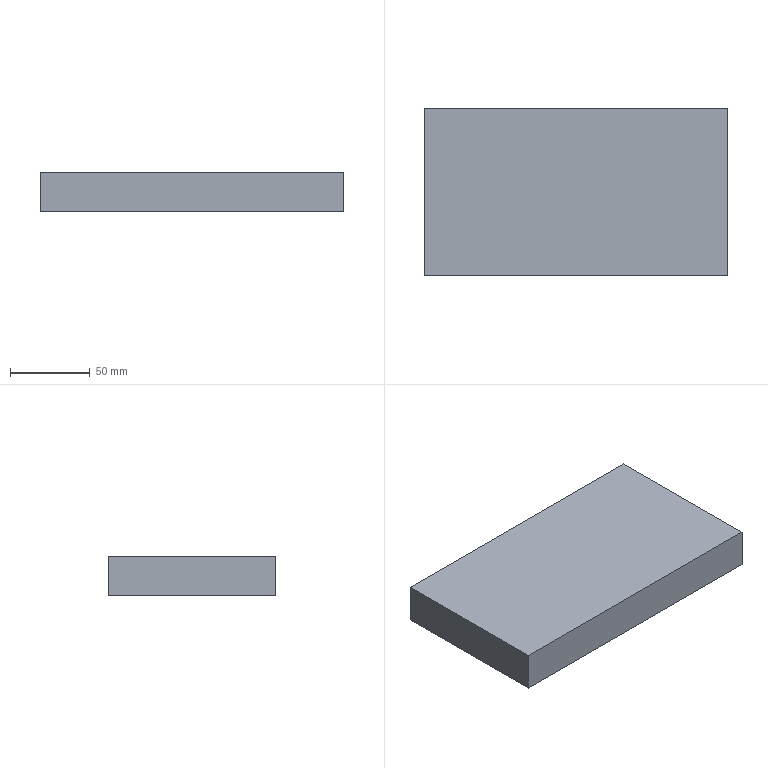Part | SolidWorks | features BaseBody 1 | 1 solid | 6 faces | box 190 x 105 x 25 mm | volume 498750 mm3 | plane 6
STEP:
#1=CARTESIAN_POINT('',(95.,-52.5,0.));
#2=VERTEX_POINT('',#1);
#3=CARTESIAN_POINT('',(95.,52.5,0.));
#4=VERTEX_POINT('',#3);
#5=CARTESIAN_POINT('',(95.,-52.5,0.));
#6=DIRECTION('',(0.,1.,0.));
#7=VECTOR('',#6,1000.);
#8=LINE('',#5,#7);
#9=EDGE_CURVE('',#2,#4,#8,.T.);
#10=ORIENTED_EDGE('',*,*,#9,.T.);
#11=CARTESIAN_POINT('',(95.,52.5,25.));
#12=VERTEX_POINT('',#11);
#13=CARTESIAN_POINT('',(95.,52.5,25.));
#14=DIRECTION('',(0.,0.,-1.));
#15=VECTOR('',#14,1000.);
#16=LINE('',#13,#15);
#17=EDGE_CURVE('',#12,#4,#16,.T.);
#18=ORIENTED_EDGE('',*,*,#17,.F.);
#19=CARTESIAN_POINT('',(95.,-52.5,25.));
#20=VERTEX_POINT('',#19);
#21=CARTESIAN_POINT('',(95.,-52.5,25.));
#22=DIRECTION('',(0.,1.,0.));
#23=VECTOR('',#22,1000.);
#24=LINE('',#21,#23);
#25=EDGE_CURVE('',#20,#12,#24,.T.);
#26=ORIENTED_EDGE('',*,*,#25,.F.);
#27=CARTESIAN_POINT('',(95.,-52.5,25.));
#28=DIRECTION('',(0.,0.,-1.));
#29=VECTOR('',#28,1000.);
#30=LINE('',#27,#29);
#31=EDGE_CURVE('',#20,#2,#30,.T.);
#32=ORIENTED_EDGE('',*,*,#31,.T.);
#33=EDGE_LOOP('',(#10,#18,#26,#32));
#34=FACE_OUTER_BOUND('',#33,.T.);
#35=CARTESIAN_POINT('',(95.,-52.5,25.));
#36=DIRECTION('',(-1.,0.,0.));
#37=DIRECTION('',(0.,0.,1.));
#38=AXIS2_PLACEMENT_3D('',#35,#36,#37);
#39=PLANE('',#38);
#40=ADVANCED_FACE('',(#34),#39,.F.);
#41=CARTESIAN_POINT('',(-95.,52.5,0.));
#42=VERTEX_POINT('',#41);
#43=CARTESIAN_POINT('',(-95.,52.5,0.));
#44=DIRECTION('',(-1.,0.,0.));
#45=VECTOR('',#44,1000.);
#46=LINE('',#43,#45);
#47=EDGE_CURVE('',#4,#42,#46,.T.);
#48=ORIENTED_EDGE('',*,*,#47,.T.);
#49=CARTESIAN_POINT('',(-95.,52.5,25.));
#50=VERTEX_POINT('',#49);
#51=CARTESIAN_POINT('',(-95.,52.5,25.));
#52=DIRECTION('',(0.,0.,-1.));
#53=VECTOR('',#52,1000.);
#54=LINE('',#51,#53);
#55=EDGE_CURVE('',#50,#42,#54,.T.);
#56=ORIENTED_EDGE('',*,*,#55,.F.);
#57=CARTESIAN_POINT('',(-95.,52.5,25.));
#58=DIRECTION('',(-1.,0.,0.));
#59=VECTOR('',#58,1000.);
#60=LINE('',#57,#59);
#61=EDGE_CURVE('',#12,#50,#60,.T.);
#62=ORIENTED_EDGE('',*,*,#61,.F.);
#63=ORIENTED_EDGE('',*,*,#17,.T.);
#64=EDGE_LOOP('',(#48,#56,#62,#63));
#65=FACE_OUTER_BOUND('',#64,.T.);
#66=CARTESIAN_POINT('',(-95.,52.5,25.));
#67=DIRECTION('',(0.,-1.,0.));
#68=DIRECTION('',(0.,0.,-1.));
#69=AXIS2_PLACEMENT_3D('',#66,#67,#68);
#70=PLANE('',#69);
#71=ADVANCED_FACE('',(#65),#70,.F.);
#72=CARTESIAN_POINT('',(-95.,-52.5,0.));
#73=VERTEX_POINT('',#72);
#74=CARTESIAN_POINT('',(-95.,-52.5,0.));
#75=DIRECTION('',(0.,-1.,0.));
#76=VECTOR('',#75,1000.);
#77=LINE('',#74,#76);
#78=EDGE_CURVE('',#42,#73,#77,.T.);
#79=ORIENTED_EDGE('',*,*,#78,.T.);
#80=CARTESIAN_POINT('',(-95.,-52.5,25.));
#81=VERTEX_POINT('',#80);
#82=CARTESIAN_POINT('',(-95.,-52.5,25.));
#83=DIRECTION('',(0.,0.,-1.));
#84=VECTOR('',#83,1000.);
#85=LINE('',#82,#84);
#86=EDGE_CURVE('',#81,#73,#85,.T.);
#87=ORIENTED_EDGE('',*,*,#86,.F.);
#88=CARTESIAN_POINT('',(-95.,-52.5,25.));
#89=DIRECTION('',(0.,-1.,0.));
#90=VECTOR('',#89,1000.);
#91=LINE('',#88,#90);
#92=EDGE_CURVE('',#50,#81,#91,.T.);
#93=ORIENTED_EDGE('',*,*,#92,.F.);
#94=ORIENTED_EDGE('',*,*,#55,.T.);
#95=EDGE_LOOP('',(#79,#87,#93,#94));
#96=FACE_OUTER_BOUND('',#95,.T.);
#97=CARTESIAN_POINT('',(-95.,-52.5,25.));
#98=DIRECTION('',(1.,0.,0.));
#99=DIRECTION('',(0.,0.,-1.));
#100=AXIS2_PLACEMENT_3D('',#97,#98,#99);
#101=PLANE('',#100);
#102=ADVANCED_FACE('',(#96),#101,.F.);
#103=CARTESIAN_POINT('',(-95.,-52.5,0.));
#104=DIRECTION('',(1.,0.,0.));
#105=VECTOR('',#104,1000.);
#106=LINE('',#103,#105);
#107=EDGE_CURVE('',#73,#2,#106,.T.);
#108=ORIENTED_EDGE('',*,*,#107,.T.);
#109=ORIENTED_EDGE('',*,*,#31,.F.);
#110=CARTESIAN_POINT('',(-95.,-52.5,25.));
#111=DIRECTION('',(1.,0.,0.));
#112=VECTOR('',#111,1000.);
#113=LINE('',#110,#112);
#114=EDGE_CURVE('',#81,#20,#113,.T.);
#115=ORIENTED_EDGE('',*,*,#114,.F.);
#116=ORIENTED_EDGE('',*,*,#86,.T.);
#117=EDGE_LOOP('',(#108,#109,#115,#116));
#118=FACE_OUTER_BOUND('',#117,.T.);
#119=CARTESIAN_POINT('',(-95.,-52.5,25.));
#120=DIRECTION('',(0.,1.,0.));
#121=DIRECTION('',(0.,0.,1.));
#122=AXIS2_PLACEMENT_3D('',#119,#120,#121);
#123=PLANE('',#122);
#124=ADVANCED_FACE('',(#118),#123,.F.);
#125=ORIENTED_EDGE('',*,*,#25,.T.);
#126=ORIENTED_EDGE('',*,*,#61,.T.);
#127=ORIENTED_EDGE('',*,*,#92,.T.);
#128=ORIENTED_EDGE('',*,*,#114,.T.);
#129=EDGE_LOOP('',(#125,#126,#127,#128));
#130=FACE_OUTER_BOUND('',#129,.T.);
#131=CARTESIAN_POINT('',(0.,0.,25.));
#132=DIRECTION('',(0.,0.,-1.));
#133=DIRECTION('',(-1.,0.,0.));
#134=AXIS2_PLACEMENT_3D('',#131,#132,#133);
#135=PLANE('',#134);
#136=ADVANCED_FACE('',(#130),#135,.F.);
#137=ORIENTED_EDGE('',*,*,#9,.F.);
#138=ORIENTED_EDGE('',*,*,#107,.F.);
#139=ORIENTED_EDGE('',*,*,#78,.F.);
#140=ORIENTED_EDGE('',*,*,#47,.F.);
#141=EDGE_LOOP('',(#137,#138,#139,#140));
#142=FACE_OUTER_BOUND('',#141,.T.);
#143=CARTESIAN_POINT('',(0.,0.,0.));
#144=DIRECTION('',(0.,0.,-1.));
#145=DIRECTION('',(-1.,0.,0.));
#146=AXIS2_PLACEMENT_3D('',#143,#144,#145);
#147=PLANE('',#146);
#148=ADVANCED_FACE('',(#142),#147,.T.);
#149=CLOSED_SHELL('',(#40,#71,#102,#124,#136,#148));
#150=MANIFOLD_SOLID_BREP('',#149);
#151=CARTESIAN_POINT('',(0.,0.,0.));
#152=DIRECTION('',(0.,0.,1.));
#153=DIRECTION('',(1.,0.,0.));
#154=AXIS2_PLACEMENT_3D('',#151,#152,#153);
#155=(LENGTH_UNIT()NAMED_UNIT(*)SI_UNIT(.MILLI.,.METRE.));
#156=UNCERTAINTY_MEASURE_WITH_UNIT(LENGTH_MEASURE(0.00001),#155,'','');
#157=(NAMED_UNIT(*)PLANE_ANGLE_UNIT()SI_UNIT($,.RADIAN.));
#158=(NAMED_UNIT(*)SI_UNIT($,.STERADIAN.)SOLID_ANGLE_UNIT());
#159=(GEOMETRIC_REPRESENTATION_CONTEXT(3)GLOBAL_UNCERTAINTY_ASSIGNED_CONTEXT((#156))GLOBAL_UNIT_ASSIGNED_CONTEXT((#155,#157,#158))REPRESENTATION_CONTEXT('',''));
#160=ADVANCED_BREP_SHAPE_REPRESENTATION('',(#150,#154),#159);